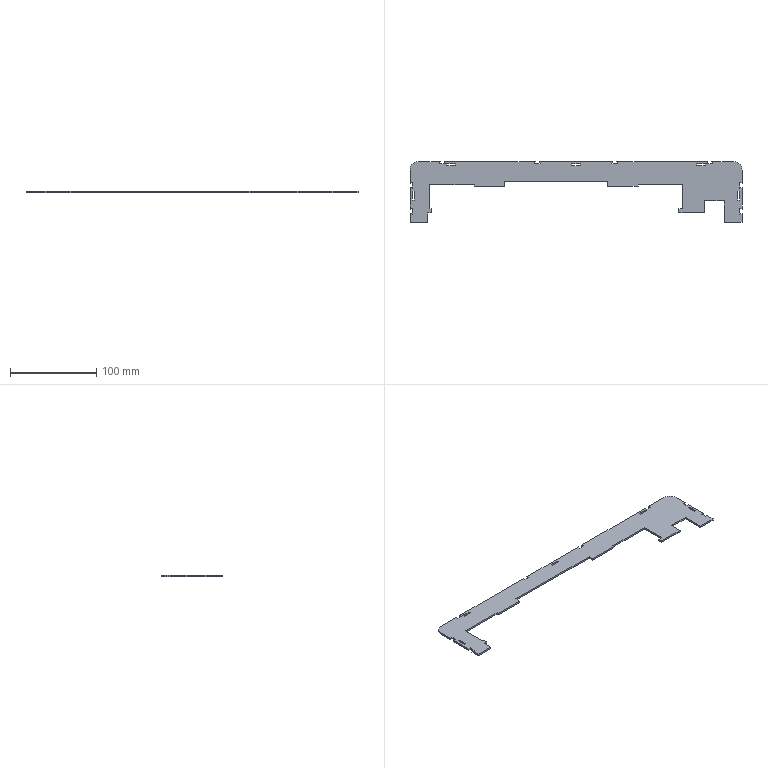Part | STEP file | xzz-003-1 | 1 solid | 82 faces | box 385.4 x 70.7 x 2 mm | volume 25743 mm3 | plane 80 | cylinder 2 | commonest cylinder face diameters 20 x2